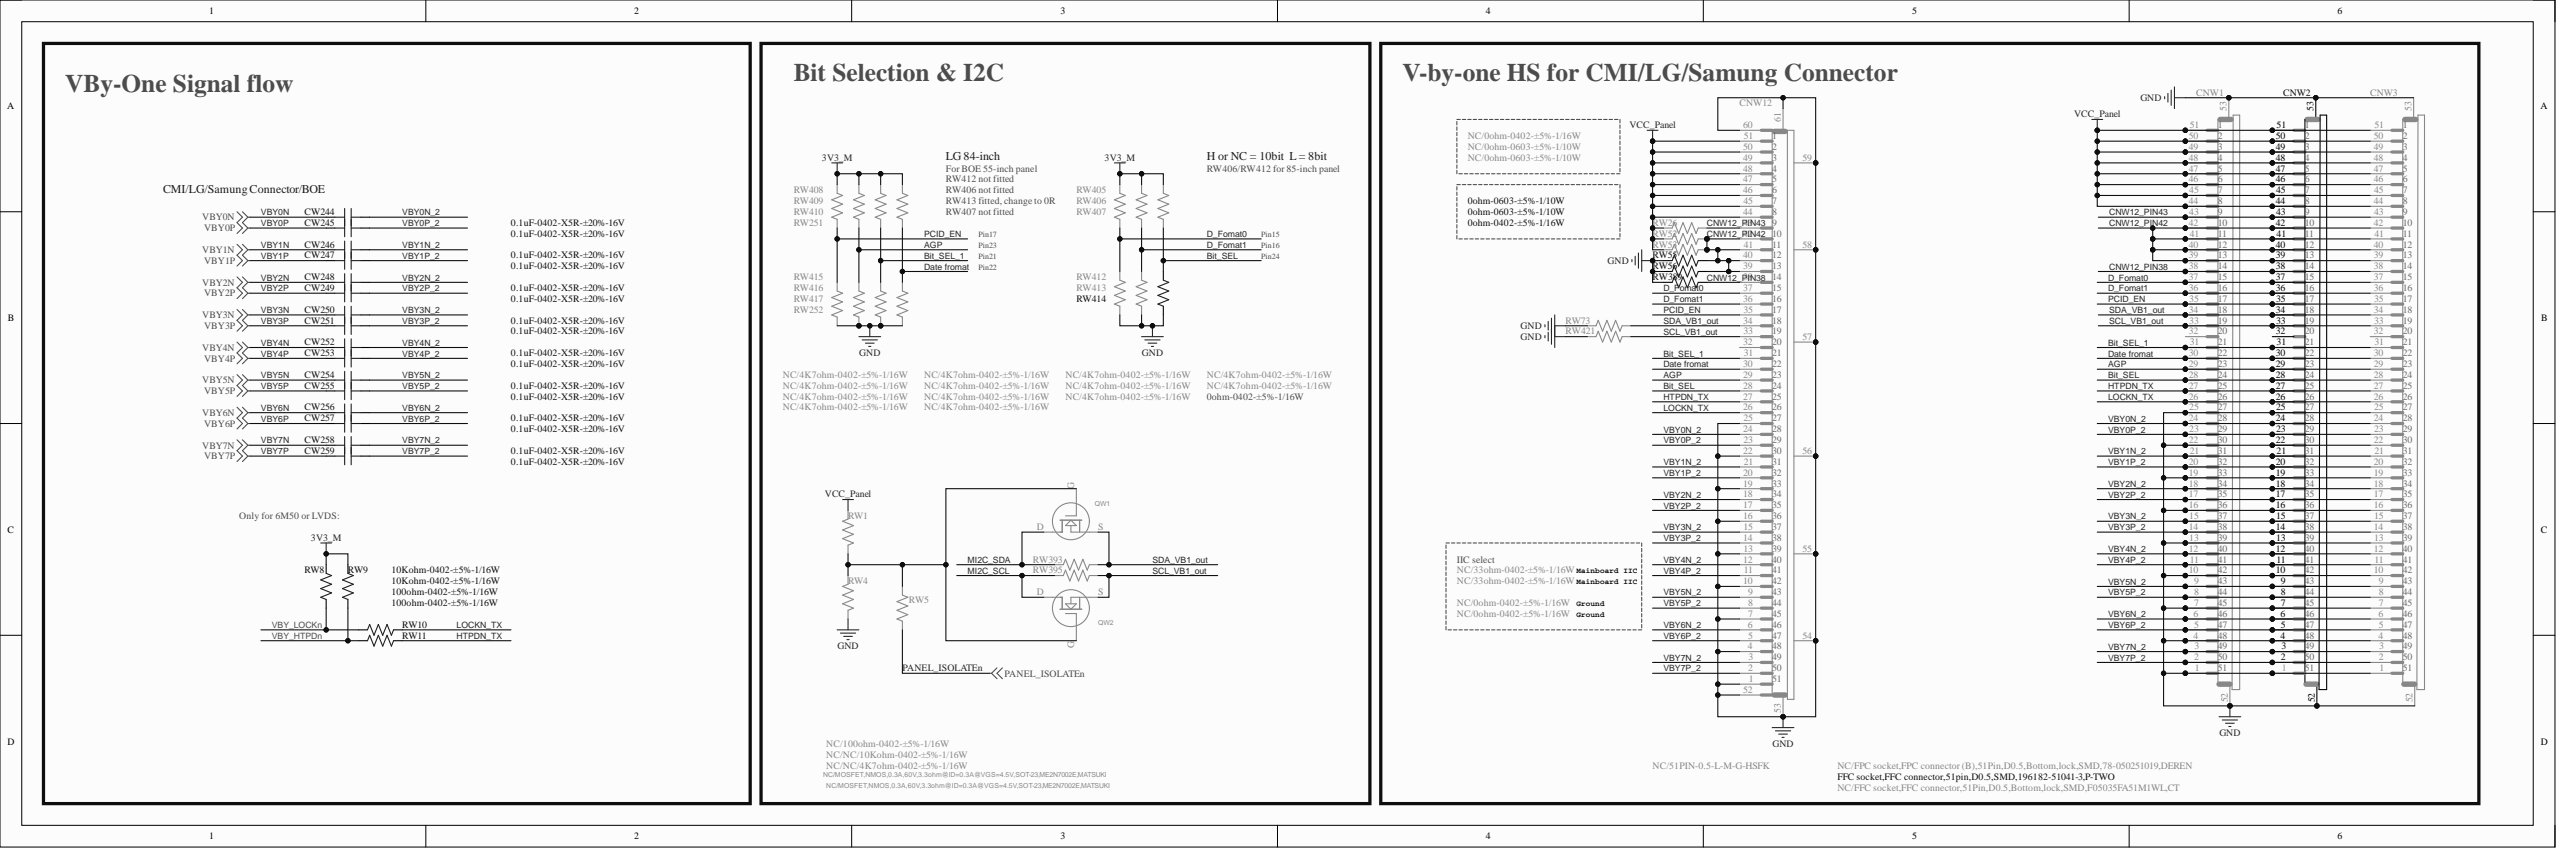Circuit board | Altium Designer | 1029 parts | 642 nets | one sheet of the schematic
Parts on this sheet (reference | value | footprint):
CNW1 | NC/FPC socket,FPC connector (B),51Pin,D0.5,Bottom,lock,SMD,78-050251019,DEREN | FFC51H/0.5S-10
CNW2 | FFC socket,FFC connector,51pin,D0.5,SMD,196182-51041-3,P-TWO | FFC51-H/0.5S-1
CNW3 | NC/FFC socket,FFC connector,51Pin,D0.5,Bottom,lock,SMD,F05035FA51M1WL,CT | FFC51H/0.5S-12
CNW12 | NC/51PIN-0.5-L-M-G-HSFK | FFC51H/0.5SA-1
CW244 | 0.1uF-0402-X5R-±20%-16V | C0402
CW245 | 0.1uF-0402-X5R-±20%-16V | C0402
CW246 | 0.1uF-0402-X5R-±20%-16V | C0402
CW247 | 0.1uF-0402-X5R-±20%-16V | C0402
CW248 | 0.1uF-0402-X5R-±20%-16V | C0402
CW249 | 0.1uF-0402-X5R-±20%-16V | C0402
CW250 | 0.1uF-0402-X5R-±20%-16V | C0402
CW251 | 0.1uF-0402-X5R-±20%-16V | C0402
CW252 | 0.1uF-0402-X5R-±20%-16V | C0402
CW253 | 0.1uF-0402-X5R-±20%-16V | C0402
CW254 | 0.1uF-0402-X5R-±20%-16V | C0402
CW255 | 0.1uF-0402-X5R-±20%-16V | C0402
CW256 | 0.1uF-0402-X5R-±20%-16V | C0402
CW257 | 0.1uF-0402-X5R-±20%-16V | C0402
CW258 | 0.1uF-0402-X5R-±20%-16V | C0402
CW259 | 0.1uF-0402-X5R-±20%-16V | C0402
QW1 | NC/MOSFET,NMOS,0.3A,60V,3.3ohm@ID=0.3A@VGS=4.5V,SOT-23,ME2N7002E,MATSUKI | SOT-23-7
QW2 | NC/MOSFET,NMOS,0.3A,60V,3.3ohm@ID=0.3A@VGS=4.5V,SOT-23,ME2N7002E,MATSUKI | SOT-23-7
RW1 | NC/NC/10Kohm-0402-±5%-1/16W | R0402
RW4 | NC/NC/4K7ohm-0402-±5%-1/16W | R0402
RW5 | NC/100ohm-0402-±5%-1/16W | R0402
RW8 | 10Kohm-0402-±5%-1/16W | R0402
RW9 | 10Kohm-0402-±5%-1/16W | R0402
RW10 | 100ohm-0402-±5%-1/16W | R0402
RW11 | 100ohm-0402-±5%-1/16W | R0402
RW26 | NC/0ohm-0402-±5%-1/16W | R0402
RW52 | NC/0ohm-0603-±5%-1/10W | R0603
RW53 | NC/0ohm-0603-±5%-1/10W | R0603
RW55 | 0ohm-0603-±5%-1/10W | R0603
RW56 | 0ohm-0603-±5%-1/10W | R0603
RW73 | NC/0ohm-0402-±5%-1/16W | R0402
RW251 | NC/4K7ohm-0402-±5%-1/16W | R0402
RW252 | NC/4K7ohm-0402-±5%-1/16W | R0402
RW389 | 0ohm-0402-±5%-1/16W | R0402
RW393 | NC/33ohm-0402-±5%-1/16W | R0402
RW395 | NC/33ohm-0402-±5%-1/16W | R0402
RW405 | NC/4K7ohm-0402-±5%-1/16W | R0402
RW406 | NC/4K7ohm-0402-±5%-1/16W | R0402
RW407 | NC/4K7ohm-0402-±5%-1/16W | R0402
RW408 | NC/4K7ohm-0402-±5%-1/16W | R0402
RW409 | NC/4K7ohm-0402-±5%-1/16W | R0402
RW410 | NC/4K7ohm-0402-±5%-1/16W | R0402
RW412 | NC/4K7ohm-0402-±5%-1/16W | R0402
RW413 | NC/4K7ohm-0402-±5%-1/16W | R0402
RW414 | 0ohm-0402-±5%-1/16W | R0402
RW415 | NC/4K7ohm-0402-±5%-1/16W | R0402
RW416 | NC/4K7ohm-0402-±5%-1/16W | R0402
RW417 | NC/4K7ohm-0402-±5%-1/16W | R0402
RW421 | NC/0ohm-0402-±5%-1/16W | R0402
Nets of these parts (net: part-pin ...):
VCC_Panel: RW1-2 RW26-2 RW52-1 RW53-1 CNW1-44 CNW1-45 CNW1-46 CNW1-47 CNW1-48 CNW1-49 CNW1-50 CNW1-51 CNW2-44 CNW2-45 CNW2-46 CNW2-47 CNW2-48 CNW2-49 CNW2-50 CNW2-51 CNW3-44 CNW3-45 CNW3-46 CNW3-47 CNW3-48 CNW3-49 CNW3-50 CNW3-51 CNW12-44 CNW12-45 CNW12-46 CNW12-47 CNW12-48 CNW12-49 CNW12-50 CNW12-51
VBY_LOCKn: RW8-2 RW10-2
VBY_HTPDn: RW9-2 RW11-2
VBY7P_2: CW259-2 CNW1-2 CNW2-2 CNW3-2 CNW12-2
VBY7P: CW259-1
VBY7N_2: CW258-2 CNW1-3 CNW2-3 CNW3-3 CNW12-3
VBY7N: CW258-1
VBY6P_2: CW257-2 CNW1-5 CNW2-5 CNW3-5 CNW12-5
VBY6P: CW257-1
VBY6N_2: CW256-2 CNW1-6 CNW2-6 CNW3-6 CNW12-6
VBY6N: CW256-1
VBY5P_2: CW255-2 CNW1-8 CNW2-8 CNW3-8 CNW12-8
VBY5P: CW255-1
VBY5N_2: CW254-2 CNW1-9 CNW2-9 CNW3-9 CNW12-9
VBY5N: CW254-1
VBY4P_2: CW253-2 CNW1-11 CNW2-11 CNW3-11 CNW12-11
VBY4P: CW253-1
VBY4N_2: CW252-2 CNW1-12 CNW2-12 CNW3-12 CNW12-12
VBY4N: CW252-1
VBY3P_2: CW251-2 CNW1-14 CNW2-14 CNW3-14 CNW12-14
VBY3P: CW251-1
VBY3N_2: CW250-2 CNW1-15 CNW2-15 CNW3-15 CNW12-15
VBY3N: CW250-1
VBY2P_2: CW249-2 CNW1-17 CNW2-17 CNW3-17 CNW12-17
VBY2P: CW249-1
VBY2N_2: CW248-2 CNW1-18 CNW2-18 CNW3-18 CNW12-18
VBY2N: CW248-1
VBY1P_2: CW247-2 CNW1-20 CNW2-20 CNW3-20 CNW12-20
VBY1P: CW247-1
VBY1N_2: CW246-2 CNW1-21 CNW2-21 CNW3-21 CNW12-21
VBY1N: CW246-1
VBY0P_2: CW245-2 CNW1-23 CNW2-23 CNW3-23 CNW12-23
VBY0P: CW245-1
VBY0N_2: CW244-2 CNW1-24 CNW2-24 CNW3-24 CNW12-24
VBY0N: CW244-1
SDA_VB1_out: QW1-S RW73-1 RW393-1 CNW1-34 CNW2-34 CNW3-34 CNW12-34
SCL_VB1_out: QW2-S RW395-1 RW421-1 CNW1-33 CNW2-33 CNW3-33 CNW12-33
PCID_EN: RW408-1 RW415-2 CNW1-35 CNW2-35 CNW3-35 CNW12-35
PANEL_ISOLATEn: RW5-1
NetQW1_G: QW1-G QW2-G RW1-1 RW4-2 RW5-2
MI2C_SDA: QW1-D RW393-2
MI2C_SCL: QW2-D RW395-2
LOCKN_TX: RW10-1 CNW1-26 CNW2-26 CNW3-26 CNW12-26
HTPDN_TX: RW11-1 CNW1-27 CNW2-27 CNW3-27 CNW12-27
GND: RW4-1 RW55-1 RW56-1 RW73-2 RW252-1 RW389-1 RW412-1 RW413-1 RW414-1 RW415-1 RW416-1 RW417-1 RW421-2 CNW1-1 CNW1-4 CNW1-7 CNW1-10 CNW1-13 CNW1-16 CNW1-19 CNW1-22 CNW1-25 CNW1-52 CNW1-53 CNW2-1 CNW2-4 CNW2-7 CNW2-10 CNW2-13 CNW2-16 CNW2-19 CNW2-22 CNW2-25 CNW2-52 CNW2-53 CNW3-1 CNW3-4 CNW3-7 CNW3-10 CNW3-13 CNW3-16 CNW3-19 CNW3-22 CNW3-25 CNW3-52 CNW3-53 CNW12-1 CNW12-4 CNW12-7 CNW12-10 CNW12-13 CNW12-16 CNW12-19 CNW12-22 CNW12-25 CNW12-52 CNW12-53 CNW12-54 CNW12-55 CNW12-56 CNW12-57 CNW12-58 CNW12-59 CNW12-60 CNW12-61
Date fromat: RW251-1 RW252-2 CNW1-30 CNW2-30 CNW3-30 CNW12-30
D_Fomat1: RW406-1 RW413-2 CNW1-36 CNW2-36 CNW3-36 CNW12-36
D_Fomat0: RW405-1 RW412-2 CNW1-37 CNW2-37 CNW3-37 CNW12-37
CNW12_PIN43: RW26-1 CNW1-43 CNW2-43 CNW3-43 CNW12-43
CNW12_PIN42: RW52-2 RW53-2 RW55-2 RW56-2 CNW1-39 CNW1-40 CNW1-41 CNW1-42 CNW2-39 CNW2-40 CNW2-41 CNW2-42 CNW3-39 CNW3-40 CNW3-41 CNW3-42 CNW12-39 CNW12-40 CNW12-41 CNW12-42
CNW12_PIN38: RW389-2 CNW1-38 CNW2-38 CNW3-38 CNW12-38
Bit_SEL_1: RW410-1 RW417-2 CNW1-31 CNW2-31 CNW3-31 CNW12-31
Bit_SEL: RW407-1 RW414-2 CNW1-28 CNW2-28 CNW3-28 CNW12-28
AGP: RW409-1 RW416-2 CNW1-29 CNW2-29 CNW3-29 CNW12-29
3V3_M: RW8-1 RW9-1 RW251-2 RW405-2 RW406-2 RW407-2 RW408-2 RW409-2 RW410-2